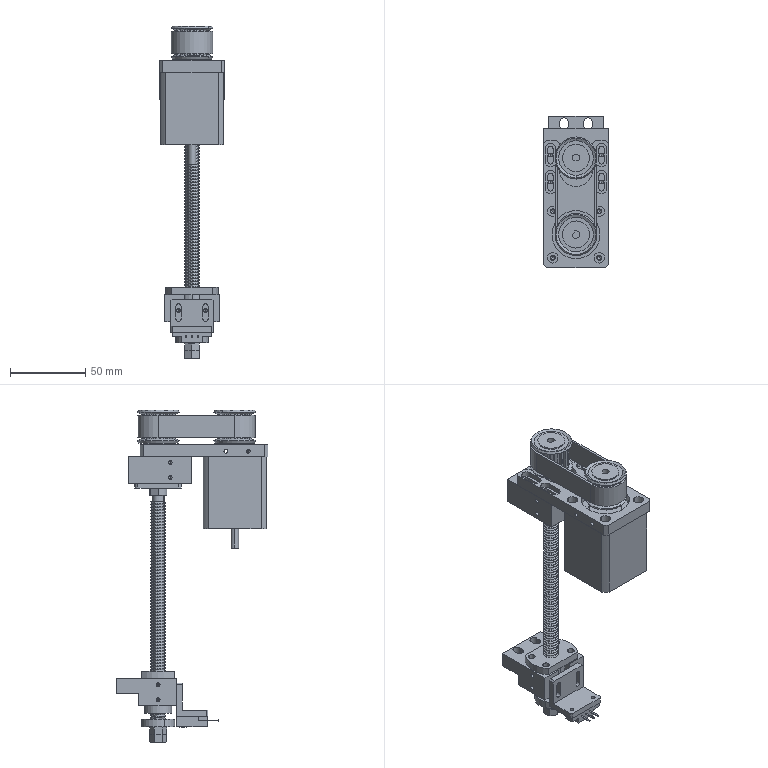Part | NX | features BREP 16 | 19 solids | 1112 faces | box 43 x 101 x 221.2 mm | volume 193277 mm3 | cylinder 493 | plane 327 | cone 169 | torus 78 | sphere 40 | spline 5 | commonest cylinder face diameters 10 x148 2.5 x50 6 x49 3.3 x32 22.91 x30 8 x26